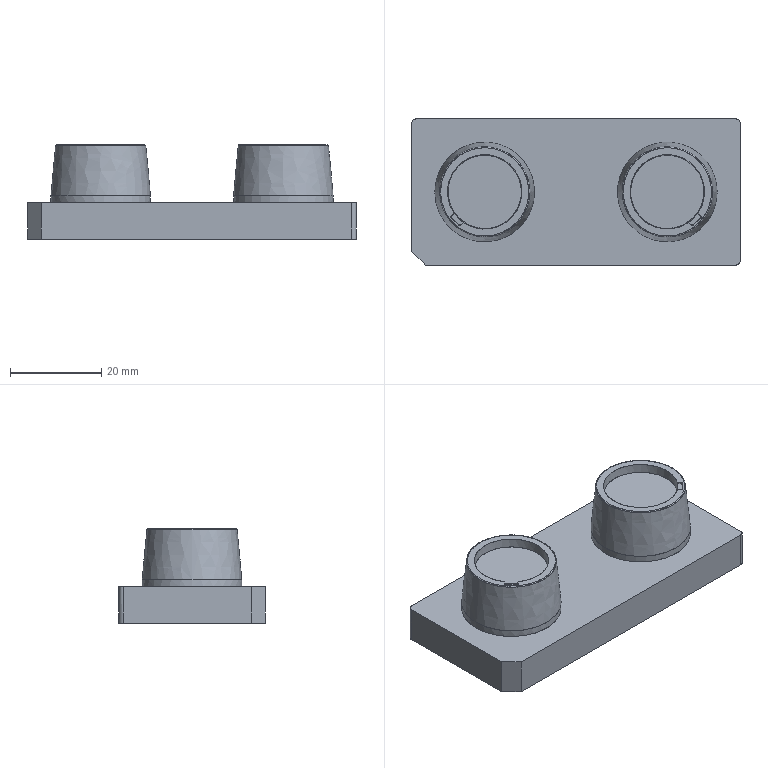NC program | PowerMill | posted with a generic post | part box 72 x 32 x 20.655 mm
Lines 25677 to 26659 of 315359:
N25774 M6
N25775 S18000 M03
N25776 G00 G90 X0.0 Y0.0
N25777 G43 Z10.805 H5
N25778
N25779 G05 P10000 R8
N25780 X21.9891 Y-11.8191
N25781 Z0.915
N25782 G01 Z-0.285 F1200.0
N25783 X21.9815 Y-11.7692 F2000.0
N25784 X21.9699 Y-11.72
N25785 X21.9545 Y-11.6719
N25786 X21.9353 Y-11.6251
N25787 X21.9125 Y-11.58
N25788 X21.8862 Y-11.5368
N25789 X21.8566 Y-11.4958
N25790 X21.8239 Y-11.4574
N25791 X21.7882 Y-11.4216
N25792 X21.7498 Y-11.3887
N25793 X21.709 Y-11.359
N25794 X21.6659 Y-11.3326
N25795 X21.6209 Y-11.3097
N25796 X21.5742 Y-11.2904
N25797 X21.5261 Y-11.2748
N25798 X21.4769 Y-11.2631
N25799 X21.427 Y-11.2553
N25800 X21.3766 Y-11.2514
N25801 X21.3261 Y-11.2516
N25802 X21.2813 Y-11.255
N25803 X21.2163 Y-11.2624
N25804 X21.1513 Y-11.2689
N25805 X21.0862 Y-11.275
N25806 X21.021 Y-11.2808
N25807 X20.9387 Y-11.2878
N25808 X20.8419 Y-11.2956
N25809 X20.7767 Y-11.3006
N25810 X20.7115 Y-11.3053
N25811 X20.6462 Y-11.3097
N25812 X20.581 Y-11.3134
N25813 X20.5156 Y-11.3158
N25814 X20.3907 Y-11.3198
N25815 X20.2657 Y-11.3239
N25816 X20.1407 Y-11.3269
N25817 X20.0158 Y-11.3281
N25818 X19.8908 Y-11.3272
N25819 X19.7658 Y-11.3247
N25820 X19.6409 Y-11.3211
N25821 X19.408 Y-11.3114
N25822 X19.1801 Y-11.298
N25823 X19.0868 Y-11.2909
N25824 X18.9936 Y-11.2825
N25825 X18.9004 Y-11.2736
N25826 X18.8073 Y-11.2641
N25827 X18.7142 Y-11.2541
N25828 X18.6212 Y-11.2436
N25829 X18.5283 Y-11.2322
N25830 X18.4356 Y-11.2191
N25831 X18.2011 Y-11.1838
N25832 X18.02 Y-11.1539
N25833 X17.8645 Y-11.125
N25834 X17.7551 Y-11.1024
N25835 X17.6458 Y-11.0797
N25836 X17.5365 Y-11.0567
N25837 X17.4276 Y-11.0319
N25838 X17.319 Y-11.0058
N25839 X17.1453 Y-10.9618
N25840 X16.9721 Y-10.9157
N25841 X16.8623 Y-10.8851
N25842 X16.7248 Y-10.8435
N25843 X16.5732 Y-10.7971
N25844 X16.4158 Y-10.7463
N25845 X16.2329 Y-10.6835
N25846 X16.0887 Y-10.6311
N25847 X15.9315 Y-10.5706
N25848 X15.867 Y-10.5454
N25849 X15.8025 Y-10.5205
N25850 X15.7379 Y-10.4956
N25851 X15.6736 Y-10.4701
N25852 X15.6099 Y-10.4431
N25853 X15.5465 Y-10.4152
N25854 X15.4016 Y-10.3514
N25855 X15.2574 Y-10.2863
N25856 X15.1689 Y-10.2448
N25857 X15.0806 Y-10.2028
N25858 X14.9925 Y-10.1603
N25859 X14.9047 Y-10.1172
N25860 X14.8174 Y-10.0732
N25861 X14.731 Y-10.0276
N25862 X14.5358 Y-9.9225
N25863 X14.3828 Y-9.8371
N25864 X14.243 Y-9.7553
N25865 X14.084 Y-9.6604
N25866 X13.9739 Y-9.5923
N25867 X13.8336 Y-9.5017
N25868 X13.6991 Y-9.4141
N25869 X13.6349 Y-9.3712
N25870 X13.5713 Y-9.3273
N25871 X13.508 Y-9.283
N25872 X13.445 Y-9.2382
N25873 X13.3822 Y-9.1933
N25874 X13.3195 Y-9.148
N25875 X13.2571 Y-9.1025
N25876 X13.1164 Y-8.9967
N25877 X12.9642 Y-8.8776
N25878 X12.8145 Y-8.7565
N25879 X12.676 Y-8.6411
N25880 X12.5145 Y-8.5019
N25881 X12.3661 Y-8.3694
N25882 X12.2363 Y-8.2492
N25883 X12.0894 Y-8.1081
N25884 X11.9789 Y-7.9994
N25885 X11.865 Y-7.8832
N25886 X11.7163 Y-7.727
N25887 X11.6507 Y-7.6574
N25888 X11.5787 Y-7.5778
N25889 X11.5307 Y-7.5241
N25890 X11.4834 Y-7.4697
N25891 X11.4365 Y-7.415
N25892 X11.3898 Y-7.3601
N25893 X11.3305 Y-7.2898
N25894 X11.2841 Y-7.2346
N25895 X11.238 Y-7.1792
N25896 X11.1921 Y-7.1237
N25897 X11.1469 Y-7.0675
N25898 X11.0267 Y-6.9136
N25899 X10.9052 Y-6.7535
N25900 X10.8155 Y-6.6314
N25901 X10.7281 Y-6.5078
N25902 X10.6423 Y-6.383
N25903 X10.5579 Y-6.2572
N25904 X10.4748 Y-6.1305
N25905 X10.3932 Y-6.003
N25906 X10.3437 Y-5.9238
N25907 X10.2955 Y-5.8437
N25908 X10.2481 Y-5.7633
N25909 X10.2012 Y-5.6825
N25910 X10.1505 Y-5.5939
N25911 X10.1044 Y-5.5126
N25912 X10.0589 Y-5.4311
N25913 X10.0139 Y-5.3492
N25914 X9.97 Y-5.2668
N25915 X9.9275 Y-5.1837
N25916 X9.8653 Y-5.0613
N25917 X9.8048 Y-4.938
N25918 X9.7284 Y-4.7753
N25919 X9.6305 Y-4.5604
N25920 X9.5947 Y-4.4781
N25921 X9.5432 Y-4.3528
N25922 X9.5105 Y-4.2769
N25923 X9.4879 Y-4.2231
N25924 X9.467 Y-4.1685
N25925 X9.4213 Y-4.0493
N25926 X9.3759 Y-3.93
N25927 X9.3315 Y-3.8103
N25928 X9.289 Y-3.69
N25929 X9.2487 Y-3.5689
N25930 X9.21 Y-3.4474
N25931 X9.1721 Y-3.3255
N25932 X9.1222 Y-3.1603
N25933 X9.0752 Y-2.9942
N25934 X9.0482 Y-2.896
N25935 X9.0228 Y-2.7974
N25936 X8.9989 Y-2.6983
N25937 X8.9747 Y-2.5994
N25938 X8.961 Y-2.5396
N25939 X8.9429 Y-2.4549
N25940 X8.8997 Y-2.2577
N25941 X8.8708 Y-2.1157
N25942 X8.8488 Y-1.9917
N25943 X8.8065 Y-1.7334
N25944 X8.796 Y-1.6698
N25945 X8.7865 Y-1.606
N25946 X8.7778 Y-1.5421
N25947 X8.7696 Y-1.4782
N25948 X8.7611 Y-1.4101
N25949 X8.7508 Y-1.3246
N25950 X8.7433 Y-1.2605
N25951 X8.7361 Y-1.1965
N25952 X8.7294 Y-1.1323
N25953 X8.7236 Y-1.0681
N25954 X8.712 Y-0.9307
N25955 X8.7008 Y-0.7932
N25956 X8.6913 Y-0.6556
N25957 X8.6846 Y-0.5179
N25958 X8.68 Y-0.38
N25959 X8.6763 Y-0.2422
N25960 X8.6735 Y-0.098
N25961 X8.6732 Y0.0461
N25962 X8.6753 Y0.1903
N25963 X8.6777 Y0.3146
N25964 X8.681 Y0.439
N25965 X8.6865 Y0.5632
N25966 X8.694 Y0.6873
N25967 X8.7025 Y0.8114
N25968 X8.7114 Y0.9354
N25969 X8.7261 Y1.0971
N25970 X8.7478 Y1.2974
N25971 X8.7646 Y1.4431
N25972 X8.777 Y1.5394
N25973 X8.791 Y1.6355
N25974 X8.8058 Y1.7315
N25975 X8.8218 Y1.8303
N25976 X8.8378 Y1.9261
N25977 X8.8544 Y2.0218
N25978 X8.8717 Y2.1174
N25979 X8.8902 Y2.2127
N25980 X8.9377 Y2.4359
N25981 X8.9881 Y2.654
N25982 X9.0412 Y2.8665
N25983 X9.0853 Y3.031
N25984 X9.132 Y3.1948
N25985 X9.1811 Y3.3578
N25986 X9.2325 Y3.5202
N25987 X9.2864 Y3.6817
N25988 X9.3433 Y3.8423
N25989 X9.4027 Y4.0019
N25990 X9.4771 Y4.1941
N25991 X9.5321 Y4.3296
N25992 X9.5863 Y4.456
N25993 X9.6649 Y4.6343
N25994 X9.7042 Y4.7243
N25995 X9.7517 Y4.8254
N25996 X9.8137 Y4.9531
N25997 X9.8749 Y5.0796
N25998 X9.9376 Y5.2054
N25999 X9.9796 Y5.2857
N26000 X10.023 Y5.3654
N26001 X10.0669 Y5.4447
N26002 X10.1116 Y5.5246
N26003 X10.1561 Y5.6036
N26004 X10.201 Y5.6824
N26005 X10.2466 Y5.7608
N26006 X10.294 Y5.8401
N26007 X10.3898 Y5.997
N26008 X10.4885 Y6.1521
N26009 X10.5714 Y6.2793
N26010 X10.6566 Y6.405
N26011 X10.7434 Y6.5296
N26012 X10.8318 Y6.6531
N26013 X10.9217 Y6.7754
N26014 X11.044 Y6.9358
N26015 X11.1748 Y7.101
N26016 X11.3153 Y7.2723
N26017 X11.4289 Y7.4067
N26018 X11.539 Y7.5326
N26019 X11.6541 Y7.6594
N26020 X11.7856 Y7.8
N26021 X11.9012 Y7.9209
N26022 X11.9671 Y7.9878
N26023 X12.0338 Y8.0539
N26024 X12.101 Y8.1196
N26025 X12.1686 Y8.1848
N26026 X12.2367 Y8.2495
N26027 X12.3053 Y8.3136
N26028 X12.3747 Y8.3768
N26029 X12.5092 Y8.4971
N26030 X12.6453 Y8.6156
N26031 X12.7837 Y8.7314
N26032 X12.9236 Y8.8453
N26033 X13.0541 Y8.9486
N26034 X13.1866 Y9.0495
N26035 X13.3206 Y9.1484
N26036 X13.4558 Y9.2455
N26037 X13.5825 Y9.334
N26038 X13.7339 Y9.4377
N26039 X13.8004 Y9.482
N26040 X13.8924 Y9.5394
N26041 X13.9688 Y9.5876
N26042 X14.0488 Y9.6396
N26043 X14.0702 Y9.6518
N26044 X14.0961 Y9.6665
N26045 X14.1607 Y9.7065
N26046 X14.2311 Y9.7494
N26047 X14.3151 Y9.7979
N26048 X14.4204 Y9.8575
N26049 X14.5262 Y9.9165
N26050 X14.5768 Y9.9449
N26051 X14.6278 Y9.9724
N26052 X14.6791 Y9.9996
N26053 X14.7304 Y10.0266
N26054 X14.8031 Y10.0645
N26055 X14.8546 Y10.0911
N26056 X14.9062 Y10.1176
N26057 X14.9579 Y10.1439
N26058 X15.01 Y10.1695
N26059 X15.1232 Y10.2233
N26060 X15.2281 Y10.2723
N26061 X15.3333 Y10.3206
N26062 X15.4389 Y10.3681
N26063 X15.5448 Y10.4147
N26064 X15.6516 Y10.4595
N26065 X15.8216 Y10.5284
N26066 X15.9805 Y10.5901
N26067 X16.1199 Y10.6415
N26068 X16.2597 Y10.692
N26069 X16.4002 Y10.7404
N26070 X16.5413 Y10.7871
N26071 X16.6944 Y10.835
N26072 X16.8442 Y10.8789
N26073 X16.9943 Y10.9215
N26074 X17.1453 Y10.9609
N26075 X17.2655 Y10.9916
N26076 X17.3858 Y11.0216
N26077 X17.5066 Y11.0496
N26078 X17.6206 Y11.0737
N26079 X17.7347 Y11.0978
N26080 X17.8489 Y11.1217
N26081 X17.9634 Y11.1439
N26082 X18.0782 Y11.1638
N26083 X18.1933 Y11.1824
N26084 X18.3085 Y11.2002
N26085 X18.491 Y11.2255
N26086 X18.6578 Y11.2466
N26087 X18.702 Y11.252
N26088 X18.7117 Y11.2543
N26089 X18.7216 Y11.2562
N26090 X18.778 Y11.2612
N26091 X18.8462 Y11.2672
N26092 X18.9385 Y11.2768
N26093 X19.031 Y11.2851
N26094 X19.1235 Y11.2923
N26095 X19.2161 Y11.299
N26096 X19.3214 Y11.306
N26097 X19.414 Y11.3116
N26098 X19.5067 Y11.3164
N26099 X19.5995 Y11.32
N26100 X19.7857 Y11.3246
N26101 X19.8865 Y11.3266
N26102 X19.9873 Y11.3271
N26103 X20.0881 Y11.3265
N26104 X20.1889 Y11.3252
N26105 X20.2897 Y11.3232
N26106 X20.3904 Y11.3207
N26107 X20.4912 Y11.3171
N26108 X20.5918 Y11.3119
N26109 X20.7858 Y11.3005
N26110 X20.93 Y11.2896
N26111 X21.0587 Y11.2771
N26112 X21.2163 Y11.2619
N26113 X21.3159 Y11.2507
N26114 X21.4153 Y11.2374
N26115 X21.5556 Y11.2206
N26116 X21.6432 Y11.209
N26117 X21.7304 Y11.1949
N26118 X21.8466 Y11.1751
N26119 X21.9628 Y11.1554
N26120 X22.0788 Y11.1346
N26121 X22.1946 Y11.1125
N26122 X22.3885 Y11.0725
N26123 X22.6022 Y11.0246
N26124 X22.7257 Y10.9944
N26125 X22.858 Y10.961
N26126 X22.9732 Y10.9309
N26127 X23.0879 Y10.8986
N26128 X23.2066 Y10.8637
N26129 X23.3206 Y10.8289
N26130 X23.4342 Y10.793
N26131 X23.5476 Y10.7564
N26132 X23.7062 Y10.704
N26133 X23.8636 Y10.6482
N26134 X24.0201 Y10.5897
N26135 X24.0924 Y10.5624
N26136 X24.1644 Y10.5342
N26137 X24.2362 Y10.5053
N26138 X24.3079 Y10.4763
N26139 X24.3794 Y10.4469
N26140 X24.4508 Y10.4171
N26141 X24.5217 Y10.3863
N26142 X24.7266 Y10.2941
N26143 X24.9188 Y10.2037
N26144 X25.1002 Y10.1142
N26145 X25.2313 Y10.0473
N26146 X25.3615 Y9.9786
N26147 X25.4907 Y9.908
N26148 X25.6192 Y9.8362
N26149 X25.7579 Y9.7548
N26150 X25.891 Y9.6748
N26151 X26.0524 Y9.5756
N26152 X26.1831 Y9.4919
N26153 X26.3123 Y9.4058
N26154 X26.4773 Y9.293
N26155 X26.5795 Y9.2203
N26156 X26.6679 Y9.1573
N26157 X26.7321 Y9.1108
N26158 X26.7955 Y9.0633
N26159 X26.8586 Y9.0154
N26160 X26.9214 Y8.967
N26161 X26.9839 Y8.9184
N26162 X27.0462 Y8.8693
N26163 X27.1079 Y8.8197
N26164 X27.2769 Y8.6811
N26165 X27.409 Y8.5693
N26166 X27.5052 Y8.4847
N26167 X27.5832 Y8.4148
N26168 X27.6611 Y8.3449
N26169 X27.7379 Y8.2737
N26170 X27.8136 Y8.2014
N26171 X27.8889 Y8.1286
N26172 X28.0035 Y8.0164
N26173 X28.1161 Y7.9022
N26174 X28.2362 Y7.7772
N26175 X28.3629 Y7.6409
N26176 X28.4912 Y7.498
N26177 X28.5726 Y7.405
N26178 X28.6529 Y7.3112
N26179 X28.7316 Y7.2159
N26180 X28.8097 Y7.1201
N26181 X28.8873 Y7.024
N26182 X28.9892 Y6.8934
N26183 X29.089 Y6.761
N26184 X29.1793 Y6.6385
N26185 X29.2193 Y6.5826
N26186 X29.2586 Y6.5263
N26187 X29.2977 Y6.4699
N26188 X29.3366 Y6.4132
N26189 X29.393 Y6.3305
N26190 X29.4315 Y6.2736
N26191 X29.4698 Y6.2166
N26192 X29.5078 Y6.1594
N26193 X29.5453 Y6.1018
N26194 X29.5816 Y6.0435
N26195 X29.6939 Y5.8592
N26196 X29.8039 Y5.6735
N26197 X29.8877 Y5.5275
N26198 X29.9704 Y5.3767
N26199 X30.0642 Y5.1986
N26200 X30.1499 Y5.0298
N26201 X30.2301 Y4.8639
N26202 X30.3069 Y4.6978
N26203 X30.387 Y4.5189
N26204 X30.4515 Y4.3675
N26205 X30.5141 Y4.2138
N26206 X30.5862 Y4.03
N26207 X30.6465 Y3.8675
N26208 X30.6926 Y3.7379
N26209 X30.7271 Y3.6364
N26210 X30.7599 Y3.5376
N26211 X30.7928 Y3.439
N26212 X30.8246 Y3.3399
N26213 X30.8547 Y3.2404
N26214 X30.8838 Y3.1405
N26215 X30.9343 Y2.9594
N26216 X30.9819 Y2.7775
N26217 X31.0264 Y2.5948
N26218 X31.0733 Y2.3866
N26219 X31.109 Y2.2142
N26220 X31.1432 Y2.0325
N26221 X31.166 Y1.9049
N26222 X31.1756 Y1.8474
N26223 X31.1848 Y1.7899
N26224 X31.1938 Y1.7323
N26225 X31.2047 Y1.6608
N26226 X31.2132 Y1.6031
N26227 X31.2216 Y1.5455
N26228 X31.2297 Y1.4878
N26229 X31.2369 Y1.43
N26230 X31.256 Y1.2609
N26231 X31.274 Y1.0918
N26232 X31.2898 Y0.9224
N26233 X31.3027 Y0.7529
N26234 X31.306 Y0.6997
N26235 X31.3089 Y0.6466
N26236 X31.3116 Y0.5934
N26237 X31.3145 Y0.5334
N26238 X31.317 Y0.4802
N26239 X31.3193 Y0.4271
N26240 X31.3214 Y0.3739
N26241 X31.3232 Y0.3207
N26242 X31.3241 Y0.2675
N26243 X31.326 Y0.1245
N26244 X31.3274 Y-0.0185
N26245 X31.3263 Y-0.1614
N26246 X31.323 Y-0.3044
N26247 X31.3181 Y-0.4694
N26248 X31.3095 Y-0.6342
N26249 X31.2984 Y-0.7989
N26250 X31.2887 Y-0.9331
N26251 X31.2747 Y-1.0819
N26252 X31.2518 Y-1.2963
N26253 X31.2341 Y-1.4529
N26254 X31.2116 Y-1.6191
N26255 X31.185 Y-1.7894
N26256 X31.1612 Y-1.9346
N26257 X31.1423 Y-2.0376
N26258 X31.1135 Y-2.1853
N26259 X31.0841 Y-2.3328
N26260 X31.0525 Y-2.4799
N26261 X31.0185 Y-2.6265
N26262 X30.9867 Y-2.7596
N26263 X30.9498 Y-2.9012
N26264 X30.8977 Y-3.0889
N26265 X30.8618 Y-3.2167
N26266 X30.8211 Y-3.3513
N26267 X30.7665 Y-3.5211
N26268 X30.7054 Y-3.7022
N26269 X30.6335 Y-3.9033
N26270 X30.5922 Y-4.0146
N26271 X30.5424 Y-4.142
N26272 X30.5071 Y-4.2336
N26273 X30.4704 Y-4.3247
N26274 X30.4324 Y-4.4152
N26275 X30.3935 Y-4.5053
N26276 X30.3539 Y-4.5952
N26277 X30.3135 Y-4.6846
N26278 X30.2546 Y-4.8125
N26279 X30.1944 Y-4.9398
N26280 X30.1318 Y-5.0659
N26281 X30.0676 Y-5.1912
N26282 X30.0269 Y-5.2709
N26283 X29.9854 Y-5.3502
N26284 X29.9423 Y-5.4286
N26285 X29.8991 Y-5.507
N26286 X29.8307 Y-5.629
N26287 X29.7434 Y-5.7775
N26288 X29.6426 Y-5.9456
N26289 X29.6108 Y-5.997
N26290 X29.5784 Y-6.0479
N26291 X29.5456 Y-6.0986
N26292 X29.511 Y-6.1519
N26293 X29.4642 Y-6.2234
N26294 X29.431 Y-6.2739
N26295 X29.3976 Y-6.3242
N26296 X29.3641 Y-6.3745
N26297 X29.3308 Y-6.4233
N26298 X29.2969 Y-6.4717
N26299 X29.2629 Y-6.52
N26300 X29.2287 Y-6.5682
N26301 X29.1944 Y-6.6164
N26302 X29.16 Y-6.6644
N26303 X29.1254 Y-6.7123
N26304 X29.0902 Y-6.7598
N26305 X28.9449 Y-6.9497
N26306 X28.8269 Y-7.0994
N26307 X28.7188 Y-7.2313
N26308 X28.6262 Y-7.3423
N26309 X28.5319 Y-7.4519
N26310 X28.4358 Y-7.5599
N26311 X28.2851 Y-7.7243
N26312 X28.1366 Y-7.8808
N26313 X27.9963 Y-8.0234
N26314 X27.8551 Y-8.1616
N26315 X27.7023 Y-8.3059
N26316 X27.5347 Y-8.4588
N26317 X27.4608 Y-8.5247
N26318 X27.3857 Y-8.5894
N26319 X27.31 Y-8.6532
N26320 X27.2338 Y-8.7165
N26321 X27.1574 Y-8.7795
N26322 X27.0805 Y-8.842
N26323 X27.0032 Y-8.9038
N26324 X26.8889 Y-8.9925
N26325 X26.7735 Y-9.0796
N26326 X26.6301 Y-9.1848
N26327 X26.4851 Y-9.2877
N26328 X26.3382 Y-9.388
N26329 X26.1975 Y-9.482
N26330 X26.0554 Y-9.5738
N26331 X25.9499 Y-9.6398
N26332 X25.8587 Y-9.6954
N26333 X25.7668 Y-9.7497
N26334 X25.6744 Y-9.8033
N26335 X25.5659 Y-9.8654
N26336 X25.4728 Y-9.9177
N26337 X25.3793 Y-9.9693
N26338 X25.2851 Y-10.0195
N26339 X25.1901 Y-10.0684
N26340 X24.998 Y-10.1653
N26341 X24.8347 Y-10.2442
N26342 X24.705 Y-10.3038
N26343 X24.5748 Y-10.3621
N26344 X24.4442 Y-10.4197
N26345 X24.3126 Y-10.4749
N26346 X24.18 Y-10.5277
N26347 X24.047 Y-10.5795
N26348 X23.9025 Y-10.6347
N26349 X23.7571 Y-10.6876
N26350 X23.6105 Y-10.7373
N26351 X23.4634 Y-10.7853
N26352 X23.3159 Y-10.8319
N26353 X23.1352 Y-10.8853
N26354 X22.9357 Y-10.9403
N26355 X22.7425 Y-10.9904
N26356 X22.6281 Y-11.0182
N26357 X22.5208 Y-11.0422
N26358 X22.4215 Y-11.0655
N26359 X22.3486 Y-11.0822
N26360 X22.2754 Y-11.0975
N26361 X22.202 Y-11.112
N26362 X22.1164 Y-11.1282
N26363 X22.0428 Y-11.1417
N26364 X21.9692 Y-11.1547
N26365 X21.8954 Y-11.1672
N26366 X21.7649 Y-11.1886
N26367 X21.6342 Y-11.2088
N26368 X21.5032 Y-11.2271
N26369 X21.372 Y-11.2436
N26370 X21.2813 Y-11.255
N26371 X21.2314 Y-11.2633
N26372 X21.1824 Y-11.2755
N26373 X21.1345 Y-11.2915
N26374 X21.088 Y-11.3113
N26375 X21.0431 Y-11.3347
N26376 X21.0003 Y-11.3615
N26377 X20.9597 Y-11.3916
N26378 X20.9217 Y-11.4249
N26379 X20.8863 Y-11.461
N26380 X20.854 Y-11.4998
N26381 X20.8248 Y-11.541
N26382 X20.7989 Y-11.5844
N26383 X20.7766 Y-11.6297
N26384 X20.7578 Y-11.6766
N26385 X20.7429 Y-11.7249
N26386 X20.7318 Y-11.7742
N26387 X20.7246 Y-11.8243
N26388 X20.7214 Y-11.8747
N26389 X20.7222 Y-11.9252
N26390 X20.7262 Y-11.97
N26391 X22.004 Y-11.9232 Z-0.3232
N26392 X21.9962 Y-11.8733
N26393 X21.9844 Y-11.8241
N26394 X21.9688 Y-11.7761
N26395 X21.9494 Y-11.7294
N26396 X21.9264 Y-11.6844
N26397 X21.9 Y-11.6413
N26398 X21.8702 Y-11.6005
N26399 X21.8373 Y-11.5621
N26400 X21.8014 Y-11.5265
N26401 X21.7629 Y-11.4938
N26402 X21.722 Y-11.4642
N26403 X21.6788 Y-11.438
N26404 X21.6337 Y-11.4153
N26405 X21.5869 Y-11.3962
N26406 X21.5387 Y-11.3808
N26407 X21.4895 Y-11.3693
N26408 X21.4395 Y-11.3617
N26409 X21.3892 Y-11.358
N26410 X21.3386 Y-11.3584
N26411 X21.2938 Y-11.3621
N26412 X21.2423 Y-11.3681
N26413 X21.218 Y-11.3708
N26414 X21.0057 Y-11.3916
N26415 X20.7938 Y-11.4084
N26416 X20.5824 Y-11.4211
N26417 X20.3716 Y-11.4299
N26418 X20.1616 Y-11.4346
N26419 X19.9719 Y-11.4354
N26420 X19.8001 Y-11.4339
N26421 X19.6284 Y-11.4302
N26422 X19.4567 Y-11.4232
N26423 X19.2852 Y-11.4132
N26424 X19.1199 Y-11.4012
N26425 X18.9547 Y-11.3878
N26426 X18.7896 Y-11.3719
N26427 X18.625 Y-11.3528
N26428 X18.4606 Y-11.331
N26429 X18.2965 Y-11.3078
N26430 X18.1307 Y-11.2819
N26431 X17.9655 Y-11.2528
N26432 X17.7961 Y-11.2211
N26433 X17.6271 Y-11.1871
N26434 X17.4588 Y-11.1503
N26435 X17.3165 Y-11.1168
N26436 X17.2214 Y-11.0933
N26437 X17.1266 Y-11.0691
N26438 X17.0249 Y-11.0425
N26439 X16.9305 Y-11.0168
N26440 X16.8363 Y-10.99
N26441 X16.7426 Y-10.9615
N26442 X16.6314 Y-10.9276
N26443 X16.5201 Y-10.8936
N26444 X16.4094 Y-10.8582
N26445 X16.2992 Y-10.821
N26446 X16.1893 Y-10.7828
N26447 X16.012 Y-10.7184
N26448 X15.8196 Y-10.6444
N26449 X15.6167 Y-10.5627
N26450 X15.4426 Y-10.4892
N26451 X15.2751 Y-10.4144
N26452 X15.1188 Y-10.3415
N26453 X14.9631 Y-10.2675
N26454 X14.8091 Y-10.1899
N26455 X14.6562 Y-10.1101
N26456 X14.4867 Y-10.0193
N26457 X14.3148 Y-9.923
N26458 X14.1697 Y-9.8381
N26459 X14.0078 Y-9.7408
N26460 X13.8448 Y-9.6387
N26461 X13.6771 Y-9.529
N26462 X13.5399 Y-9.4361
N26463 X13.4039 Y-9.3415
N26464 X13.2645 Y-9.2418
N26465 X13.1311 Y-9.1436
N26466 X12.9993 Y-9.0434
N26467 X12.8733 Y-8.9437
N26468 X12.7485 Y-8.8424
N26469 X12.6247 Y-8.74
N26470 X12.5026 Y-8.6356
N26471 X12.3823 Y-8.5291
N26472 X12.2632 Y-8.4213
N26473 X12.1276 Y-8.2953
N26474 X11.9944 Y-8.1669
N26475 X11.8636 Y-8.036
N26476 X11.7346 Y-7.9032
N26477 X11.6 Y-7.7604
N26478 X11.4679 Y-7.6152
N26479 X11.3386 Y-7.4675
N26480 X11.2116 Y-7.3178
N26481 X11.102 Y-7.184
N26482 X10.9757 Y-7.0241
N26483 X10.8702 Y-6.887
N26484 X10.7549 Y-6.732
N26485 X10.6426 Y-6.5748
N26486 X10.5332 Y-6.4155
N26487 X10.4365 Y-6.27
N26488 X10.3414 Y-6.1233
N26489 X10.2486 Y-5.9753
N26490 X10.1585 Y-5.8255
N26491 X10.0706 Y-5.6745
N26492 X9.9779 Y-5.5087
N26493 X9.8815 Y-5.3286
N26494 X9.7831 Y-5.1372
N26495 X9.6902 Y-4.9487
N26496 X9.6155 Y-4.791
N26497 X9.5669 Y-4.6837
N26498 X9.5194 Y-4.5758
N26499 X9.4728 Y-4.4676
N26500 X9.4273 Y-4.3589
N26501 X9.3958 Y-4.2802
N26502 X9.369 Y-4.2137
N26503 X9.3477 Y-4.1605
N26504 X9.3271 Y-4.1069
N26505 X9.3068 Y-4.0532
N26506 X9.2843 Y-3.9932
N26507 X9.2644 Y-3.9394
N26508 X9.2446 Y-3.8855
N26509 X9.2251 Y-3.8316
N26510 X9.2058 Y-3.7775
N26511 X9.1871 Y-3.7233
N26512 X9.1154 Y-3.5072
N26513 X9.0552 Y-3.3155
N26514 X9.0028 Y-3.1366
N26515 X8.9491 Y-2.9439
N26516 X8.9224 Y-2.8405
N26517 X8.897 Y-2.7368
N26518 X8.8723 Y-2.6329
N26519 X8.8482 Y-2.5288
N26520 X8.8247 Y-2.4246
N26521 X8.8025 Y-2.3202
N26522 X8.7609 Y-2.1109
N26523 X8.7259 Y-1.9164
N26524 X8.6959 Y-1.7298
N26525 X8.6662 Y-1.5245
N26526 X8.6434 Y-1.3448
N26527 X8.6239 Y-1.1646
N26528 X8.6037 Y-0.9454
N26529 X8.5877 Y-0.7289
N26530 X8.5758 Y-0.5152
N26531 X8.5682 Y-0.3128
N26532 X8.5645 Y-0.1072
N26533 Y0.1057
N26534 X8.5675 Y0.2886
N26535 X8.5736 Y0.4684
N26536 X8.5842 Y0.6711
N26537 X8.592 Y0.792
N26538 X8.6014 Y0.9128
N26539 X8.612 Y1.0336
N26540 X8.6236 Y1.1542
N26541 X8.636 Y1.2747
N26542 X8.6495 Y1.3951
N26543 X8.6646 Y1.5153
N26544 X8.6819 Y1.6352
N26545 X8.7123 Y1.8304
N26546 X8.7452 Y2.0252
N26547 X8.7705 Y2.1628
N26548 X8.7979 Y2.2999
N26549 X8.8271 Y2.4366
N26550 X8.8575 Y2.5731
N26551 X8.8894 Y2.7093
N26552 X8.9234 Y2.8449
N26553 X8.9809 Y3.0585
N26554 X9.0361 Y3.2507
N26555 X9.0938 Y3.4384
N26556 X9.156 Y3.6296
N26557 X9.2211 Y3.8198
N26558 X9.2894 Y4.0089
N26559 X9.3177 Y4.0844
N26560 X9.3383 Y4.137
N26561 X9.3593 Y4.1895
N26562 X9.3805 Y4.2419
N26563 X9.4024 Y4.2959
N26564 X9.4348 Y4.3751
N26565 X9.4562 Y4.4274
N26566 X9.4778 Y4.4796
N26567 X9.4996 Y4.5317
N26568 X9.522 Y4.5835
N26569 X9.6123 Y4.7833
N26570 X9.67 Y4.9066
N26571 X9.7274 Y5.0251
N26572 X9.786 Y5.1431
N26573 X9.8457 Y5.2605
N26574 X9.9068 Y5.3771
N26575 X9.9647 Y5.4836
N26576 X10.0211 Y5.585
N26577 X10.0774 Y5.6863
N26578 X10.1353 Y5.7868
N26579 X10.1951 Y5.8861
N26580 X10.2558 Y5.9848
N26581 X10.3391 Y6.1191
N26582 X10.4238 Y6.2525
N26583 X10.5116 Y6.3838
N26584 X10.601 Y6.514
N26585 X10.6692 Y6.6127
N26586 X10.7387 Y6.7104
N26587 X10.8103 Y6.8066
N26588 X10.8824 Y6.9024
N26589 X10.9959 Y7.0503
N26590 X11.1117 Y7.1963
N26591 X11.2303 Y7.3402
N26592 X11.3513 Y7.4819
N26593 X11.4743 Y7.622
N26594 X11.6155 Y7.7773
N26595 X11.7583 Y7.9286
N26596 X11.9027 Y8.0758
N26597 X12.0353 Y8.2061
N26598 X12.1697 Y8.3346
N26599 X12.3062 Y8.4609
N26600 X12.4449 Y8.5848
N26601 X12.5853 Y8.7067
N26602 X12.7009 Y8.804
N26603 X12.8466 Y8.9222
N26604 X13.0016 Y9.0447
N26605 X13.163 Y9.1673
N26606 X13.3325 Y9.2911
N26607 X13.5111 Y9.4168
N26608 X13.6387 Y9.5038
N26609 X13.7677 Y9.5887
N26610 X13.898 Y9.6717
N26611 X14.0291 Y9.7532
N26612 X14.1612 Y9.8333
N26613 X14.2811 Y9.9037
N26614 X14.4022 Y9.9722
N26615 X14.524 Y10.0393
N26616 X14.6464 Y10.1053
N26617 X14.7695 Y10.1701
N26618 X14.8935 Y10.233
N26619 X15.0992 Y10.3325
N26620 X15.3041 Y10.4271
N26621 X15.508 Y10.517
N26622 X15.6055 Y10.5584
N26623 X15.7036 Y10.5984
N26624 X15.802 Y10.6374
N26625 X15.9007 Y10.6757
N26626 X15.9997 Y10.7133
N26627 X16.0989 Y10.7503
N26628 X16.1986 Y10.786
N26629 X16.2988 Y10.8201
N26630 X16.4529 Y10.8717
N26631 X16.6077 Y10.9211
N26632 X16.7632 Y10.9683
N26633 X16.949 Y11.0217
N26634 X17.1432 Y11.0734
N26635 X17.3168 Y11.1165
N26636 X17.4827 Y11.1554
N26637 X17.6491 Y11.1918
N26638 X17.8162 Y11.2251
N26639 X17.976 Y11.255
N26640 X18.1299 Y11.2821
N26641 X18.2842 Y11.3067
N26642 X18.4388 Y11.3286
N26643 X18.5938 Y11.3488
N26644 X18.7019 Y11.3624
N26645 X18.7705 Y11.37
N26646 X18.8391 Y11.3769
N26647 X18.9078 Y11.3833
N26648 X18.9812 Y11.39
N26649 X19.0499 Y11.396
N26650 X19.1187 Y11.4018
N26651 X19.1874 Y11.4074
N26652 X19.2562 Y11.4124
N26653 X19.3251 Y11.4162
N26654 X19.4937 Y11.4248
N26655 X19.6624 Y11.4308
N26656 X19.8311 Y11.4341
N26657 X19.9999 Y11.4357
N26658 X20.1786 Y11.4342
N26659 X20.3572 Y11.4299
N26660 X20.5358 Y11.423
N26661 X20.7481 Y11.4112
N26662 X20.9591 Y11.3955
N26663 X21.1689 Y11.376
N26664 X21.3773 Y11.3525
N26665 X21.5655 Y11.328
N26666 X21.7533 Y11.3008
N26667 X21.9406 Y11.2702
N26668 X22.1273 Y11.2363
N26669 X22.3134 Y11.1995
N26670 X22.5219 Y11.1544
N26671 X22.7256 Y11.1065
N26672 X22.9247 Y11.0556
N26673 X23.0667 Y11.0168
N26674 X23.2084 Y10.9771
N26675 X23.3495 Y10.9354
N26676 X23.4898 Y10.8907
N26677 X23.6296 Y10.8449
N26678 X23.8081 Y10.7839
N26679 X23.9739 Y10.7235
N26680 X24.1674 Y10.6496
N26681 X24.3597 Y10.5723
N26682 X24.5505 Y10.4916
N26683 X24.7311 Y10.4115
N26684 X24.9103 Y10.3285
N26685 X25.088 Y10.2421
N26686 X25.264 Y10.1525
N26687 X25.4385 Y10.0598
N26688 X25.6114 Y9.9644
N26689 X25.7863 Y9.8642
N26690 X25.9594 Y9.7607
N26691 X26.1323 Y9.653
N26692 X26.3014 Y9.5432
N26693 X26.4687 Y9.4307
N26694 X26.634 Y9.3153
N26695 X26.8024 Y9.1931
N26696 X26.9711 Y9.0656
N26697 X27.1403 Y8.933
N26698 X27.3099 Y8.7949
N26699 X27.4525 Y8.6747
N26700 X27.5897 Y8.5547
N26701 X27.7479 Y8.4116
N26702 X27.9034 Y8.2657
N26703 X28.0546 Y8.1183
N26704 X28.2031 Y7.9681
N26705 X28.3463 Y7.8179
N26706 X28.484 Y7.6684
N26707 X28.6253 Y7.5091
N26708 X28.765 Y7.3457
N26709 X28.9014 Y7.18
N26710 X29.0337 Y7.0131
N26711 X29.144 Y6.8685
N26712 X29.2624 Y6.7071
N26713 X29.3908 Y6.5263
N26714 X29.5052 Y6.3593
N26715 X29.6087 Y6.2019
N26716 X29.7083 Y6.0442
N26717 X29.822 Y5.8572
N26718 X29.9324 Y5.6681
N26719 X30.0197 Y5.5125
N26720 X30.1128 Y5.3392
N26721 X30.2102 Y5.1509
N26722 X30.3028 Y4.9635
N26723 X30.3907 Y4.7767
N26724 X30.4739 Y4.5906
N26725 X30.5205 Y4.4837
N26726 X30.5658 Y4.3763
N26727 X30.6095 Y4.2683
N26728 X30.6792 Y4.0911
N26729 X30.7461 Y3.9127
N26730 X30.8096 Y3.7332
N26731 X30.8699 Y3.5525
N26732 X30.9275 Y3.371
N26733 X30.9723 Y3.223
N26734 X31.0149 Y3.0743
N26735 X31.0555 Y2.9252
N26736 X31.0928 Y2.7788
N26737 X31.1289 Y2.6322
N26738 X31.163 Y2.485
N26739 X31.1943 Y2.3373
N26740 X31.2241 Y2.1892
N26741 X31.2557 Y2.0227
N26742 X31.2844 Y1.8556
N26743 X31.3103 Y1.688
N26744 X31.3341 Y1.5201
N26745 X31.3446 Y1.4431
N26746 X31.3539 Y1.3672
N26747 X31.3624 Y1.2912
N26748 X31.3705 Y1.2152
N26749 X31.3801 Y1.1231
N26750 X31.3876 Y1.047
N26751 X31.3948 Y0.9709
N26752 X31.4013 Y0.8947
N26753 X31.4106 Y0.7582
N26754 X31.4185 Y0.6216
N26755 X31.4252 Y0.485
N26756 X31.4306 Y0.3484